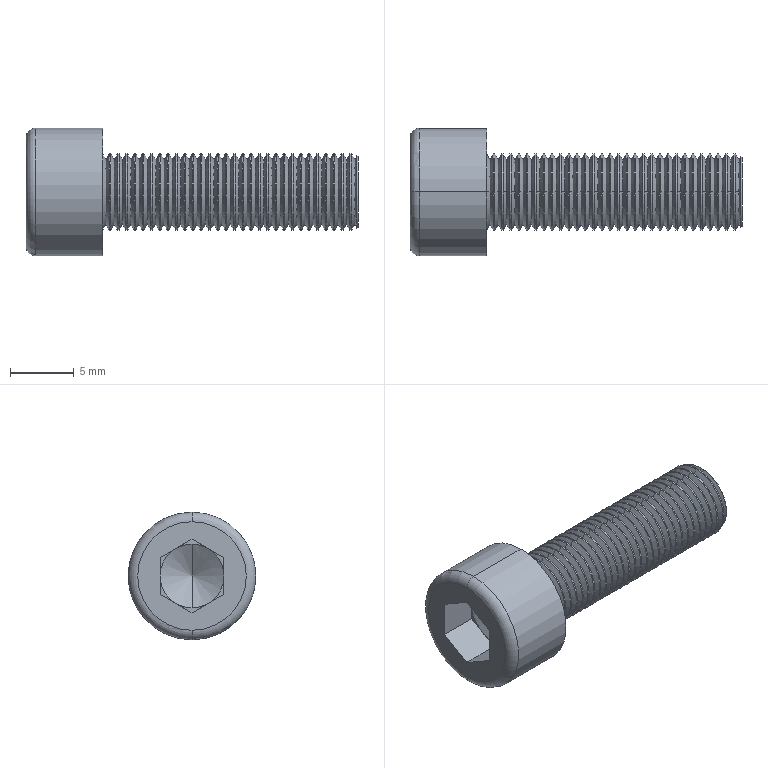Part | STEP file | PN_0037_Default<As Machined> | 1 solid | 210 faces | box 26 x 10 x 10 mm | volume 888.028 mm3 | cone 128 | cylinder 64 | plane 16 | torus 2 | commonest cylinder face diameters 6 x60 7.083 x2 10 x2